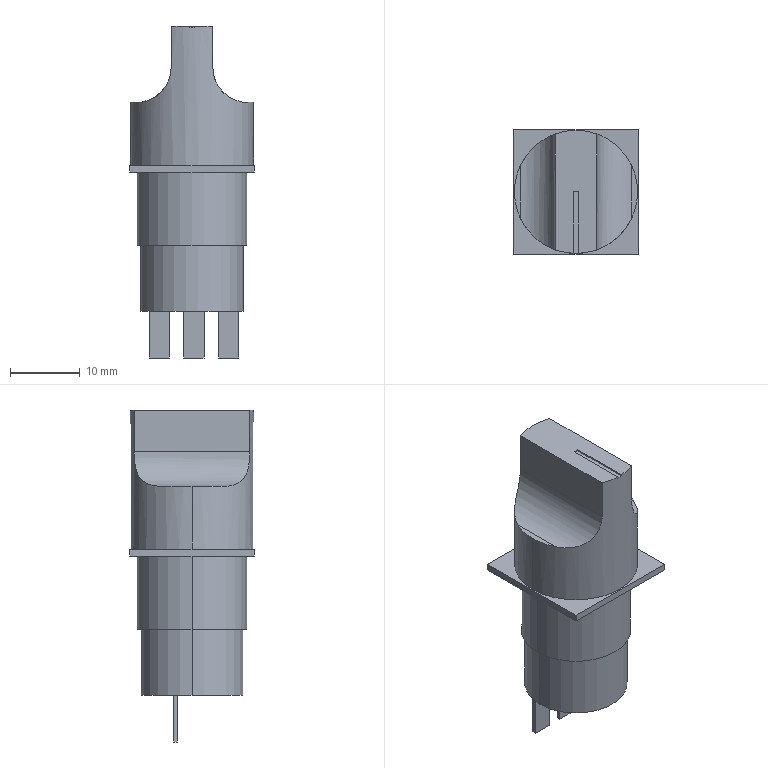Part | STEP file | 1 solid | 40 faces | box 17.9 x 17.9 x 47.75 mm | volume 7538 mm3 | plane 32 | cylinder 8 | commonest cylinder face diameters 10 x2 14.7 x2 15.77 x2 17.7 x2